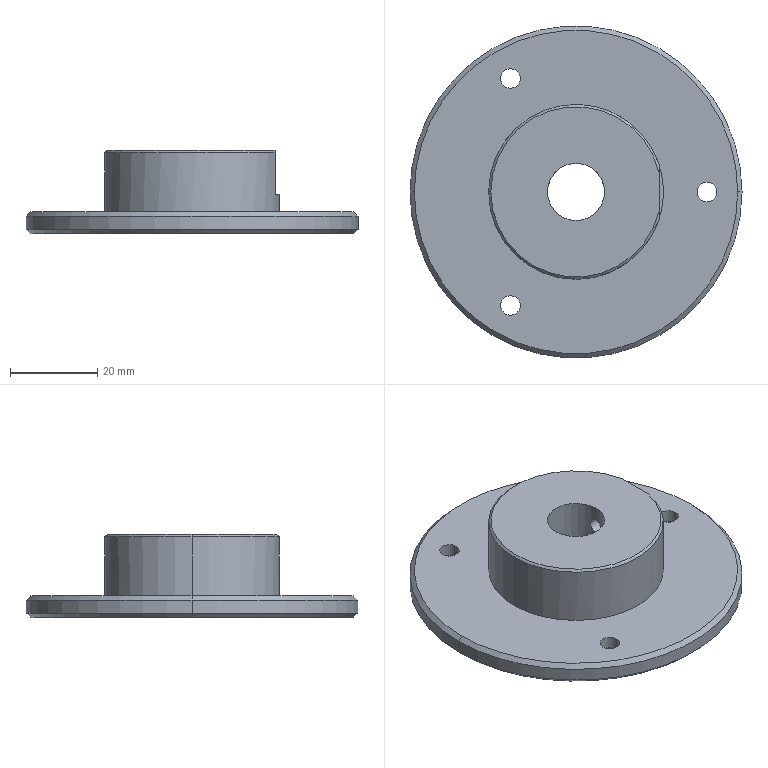Part | STEP file | 11-FG-B05411 | 1 solid | 31 faces | box 76 x 76 x 19 mm | volume 36918 mm3 | cylinder 14 | cone 12 | plane 5 | commonest cylinder face diameters 4.5 x6 3.3 x2 13.1 x2 40 x2 76 x2
STEP:
#1=CARTESIAN_POINT('',(-19.5,0.,19.));
#2=VERTEX_POINT('',#1);
#3=CARTESIAN_POINT('',(19.,-4.387,19.));
#4=VERTEX_POINT('',#3);
#5=CARTESIAN_POINT('',(0.,0.,19.));
#6=DIRECTION('',(0.,0.,1.));
#7=DIRECTION('',(1.,0.,0.));
#8=AXIS2_PLACEMENT_3D('',#5,#6,#7);
#9=CIRCLE('',#8,19.5);
#10=EDGE_CURVE('',#2,#4,#9,.T.);
#11=ORIENTED_EDGE('',*,*,#10,.F.);
#12=CARTESIAN_POINT('',(-20.,0.,18.5));
#13=VERTEX_POINT('',#12);
#14=CARTESIAN_POINT('',(-19.5,0.,19.));
#15=DIRECTION('',(-0.7071,0.,-0.7071));
#16=VECTOR('',#15,1000.);
#17=LINE('',#14,#16);
#18=EDGE_CURVE('',#2,#13,#17,.T.);
#19=ORIENTED_EDGE('',*,*,#18,.T.);
#20=CARTESIAN_POINT('',(19.,-6.245,18.5));
#21=VERTEX_POINT('',#20);
#22=CARTESIAN_POINT('',(0.,0.,18.5));
#23=DIRECTION('',(0.,0.,-1.));
#24=DIRECTION('',(1.,0.,0.));
#25=AXIS2_PLACEMENT_3D('',#22,#23,#24);
#26=CIRCLE('',#25,20.);
#27=EDGE_CURVE('',#21,#13,#26,.T.);
#28=ORIENTED_EDGE('',*,*,#27,.F.);
#29=CARTESIAN_POINT('',(19.,-4.387,19.));
#30=CARTESIAN_POINT('',(19.,-5.014,18.859));
#31=CARTESIAN_POINT('',(19.,-5.632,18.691));
#32=CARTESIAN_POINT('',(19.,-6.245,18.5));
#33=B_SPLINE_CURVE_WITH_KNOTS('',3,(#29,#30,#31,#32),.UNSPECIFIED.,.F.,.F.,(4,4),(0.,0.001924),.UNSPECIFIED.);
#34=EDGE_CURVE('',#4,#21,#33,.T.);
#35=ORIENTED_EDGE('',*,*,#34,.F.);
#36=EDGE_LOOP('',(#11,#19,#28,#35));
#37=FACE_OUTER_BOUND('',#36,.T.);
#38=CARTESIAN_POINT('',(0.,0.,19.));
#39=DIRECTION('',(0.,0.,-1.));
#40=DIRECTION('',(-1.,0.,0.));
#41=AXIS2_PLACEMENT_3D('',#38,#39,#40);
#42=CONICAL_SURFACE('',#41,19.5,0.7854);
#43=ADVANCED_FACE('',(#37),#42,.T.);
#44=CARTESIAN_POINT('',(6.55,0.,15.65));
#45=VERTEX_POINT('',#44);
#46=CARTESIAN_POINT('',(6.55,0.,12.35));
#47=VERTEX_POINT('',#46);
#48=CARTESIAN_POINT('',(6.55,0.,15.65));
#49=CARTESIAN_POINT('',(6.55,-0.2158,15.65));
#50=CARTESIAN_POINT('',(6.539,-0.4338,15.606));
#51=CARTESIAN_POINT('',(6.51,-0.7319,15.483));
#52=CARTESIAN_POINT('',(6.498,-0.8284,15.431));
#53=CARTESIAN_POINT('',(6.473,-1.007,15.311));
#54=CARTESIAN_POINT('',(6.459,-1.09,15.243));
#55=CARTESIAN_POINT('',(6.432,-1.242,15.091));
#56=CARTESIAN_POINT('',(6.418,-1.312,15.007));
#57=CARTESIAN_POINT('',(6.392,-1.431,14.829));
#58=CARTESIAN_POINT('',(6.38,-1.482,14.734));
#59=CARTESIAN_POINT('',(6.35,-1.607,14.433));
#60=CARTESIAN_POINT('',(6.339,-1.65,14.218));
#61=CARTESIAN_POINT('',(6.339,-1.65,13.892));
#62=CARTESIAN_POINT('',(6.342,-1.639,13.784));
#63=CARTESIAN_POINT('',(6.352,-1.597,13.572));
#64=CARTESIAN_POINT('',(6.36,-1.565,13.467));
#65=CARTESIAN_POINT('',(6.39,-1.441,13.169));
#66=CARTESIAN_POINT('',(6.418,-1.319,12.985));
#67=CARTESIAN_POINT('',(6.473,-1.016,12.682));
#68=CARTESIAN_POINT('',(6.5,-0.833,12.56));
#69=CARTESIAN_POINT('',(6.529,-0.5351,12.435));
#70=CARTESIAN_POINT('',(6.537,-0.43,12.403));
#71=CARTESIAN_POINT('',(6.547,-0.2173,12.361));
#72=CARTESIAN_POINT('',(6.55,-0.1095,12.35));
#73=CARTESIAN_POINT('',(6.55,0.,12.35));
#74=B_SPLINE_CURVE_WITH_KNOTS('',3,(#48,#49,#50,#51,#52,#53,#54,#55,#56,#57,#58,#59,#60,#61,#62,#63,#64,#65,#66,#67,#68,#69,#70,#71,#72,#73),.UNSPECIFIED.,.F.,.F.,(4,2,2,2,2,2,2,2,2,2,2,2,4),(0.00518,0.005827,0.006151,0.006474,0.006798,0.007121,0.007769,0.008092,0.008416,0.009063,0.009711,0.01003,0.01036),.UNSPECIFIED.);
#75=EDGE_CURVE('',#45,#47,#74,.T.);
#76=ORIENTED_EDGE('',*,*,#75,.F.);
#77=CARTESIAN_POINT('',(19.,0.,15.65));
#78=VERTEX_POINT('',#77);
#79=CARTESIAN_POINT('',(19.,0.,15.65));
#80=DIRECTION('',(1.,0.,0.));
#81=VECTOR('',#80,1000.);
#82=LINE('',#79,#81);
#83=EDGE_CURVE('',#45,#78,#82,.T.);
#84=ORIENTED_EDGE('',*,*,#83,.T.);
#85=CARTESIAN_POINT('',(19.,0.,12.35));
#86=VERTEX_POINT('',#85);
#87=CARTESIAN_POINT('',(19.,0.,14.));
#88=DIRECTION('',(1.,0.,0.));
#89=DIRECTION('',(0.,0.,-1.));
#90=AXIS2_PLACEMENT_3D('',#87,#88,#89);
#91=CIRCLE('',#90,1.65);
#92=EDGE_CURVE('',#78,#86,#91,.T.);
#93=ORIENTED_EDGE('',*,*,#92,.T.);
#94=CARTESIAN_POINT('',(19.,0.,12.35));
#95=DIRECTION('',(1.,0.,0.));
#96=VECTOR('',#95,1000.);
#97=LINE('',#94,#96);
#98=EDGE_CURVE('',#47,#86,#97,.T.);
#99=ORIENTED_EDGE('',*,*,#98,.F.);
#100=EDGE_LOOP('',(#76,#84,#93,#99));
#101=FACE_OUTER_BOUND('',#100,.T.);
#102=CARTESIAN_POINT('',(19.,0.,14.));
#103=DIRECTION('',(1.,0.,0.));
#104=DIRECTION('',(0.,0.,-1.));
#105=AXIS2_PLACEMENT_3D('',#102,#103,#104);
#106=CYLINDRICAL_SURFACE('',#105,1.65);
#107=ADVANCED_FACE('',(#101),#106,.F.);
#108=CARTESIAN_POINT('',(-12.75,25.981,2.05));
#109=VERTEX_POINT('',#108);
#110=CARTESIAN_POINT('',(-17.25,25.981,2.05));
#111=VERTEX_POINT('',#110);
#112=CARTESIAN_POINT('',(-15.,25.981,2.05));
#113=DIRECTION('',(0.,0.,-1.));
#114=DIRECTION('',(-1.,0.,0.));
#115=AXIS2_PLACEMENT_3D('',#112,#113,#114);
#116=CIRCLE('',#115,2.25);
#117=EDGE_CURVE('',#109,#111,#116,.T.);
#118=ORIENTED_EDGE('',*,*,#117,.F.);
#119=CARTESIAN_POINT('',(-10.7,25.981,0.));
#120=VERTEX_POINT('',#119);
#121=CARTESIAN_POINT('',(-10.7,25.981,0.));
#122=DIRECTION('',(0.7071,0.,-0.7071));
#123=VECTOR('',#122,1000.);
#124=LINE('',#121,#123);
#125=EDGE_CURVE('',#109,#120,#124,.T.);
#126=ORIENTED_EDGE('',*,*,#125,.T.);
#127=CARTESIAN_POINT('',(-19.3,25.981,0.));
#128=VERTEX_POINT('',#127);
#129=CARTESIAN_POINT('',(-15.,25.981,0.));
#130=DIRECTION('',(0.,0.,-1.));
#131=DIRECTION('',(-1.,0.,0.));
#132=AXIS2_PLACEMENT_3D('',#129,#130,#131);
#133=CIRCLE('',#132,4.3);
#134=EDGE_CURVE('',#120,#128,#133,.T.);
#135=ORIENTED_EDGE('',*,*,#134,.T.);
#136=CARTESIAN_POINT('',(-19.3,25.981,0.));
#137=DIRECTION('',(-0.7071,0.,-0.7071));
#138=VECTOR('',#137,1000.);
#139=LINE('',#136,#138);
#140=EDGE_CURVE('',#111,#128,#139,.T.);
#141=ORIENTED_EDGE('',*,*,#140,.F.);
#142=EDGE_LOOP('',(#118,#126,#135,#141));
#143=FACE_OUTER_BOUND('',#142,.T.);
#144=CARTESIAN_POINT('',(-15.,25.981,0.));
#145=DIRECTION('',(0.,0.,-1.));
#146=DIRECTION('',(-1.,0.,0.));
#147=AXIS2_PLACEMENT_3D('',#144,#145,#146);
#148=CONICAL_SURFACE('',#147,4.3,0.7854);
#149=ADVANCED_FACE('',(#143),#148,.F.);
#150=CARTESIAN_POINT('',(-17.25,25.981,5.));
#151=VERTEX_POINT('',#150);
#152=CARTESIAN_POINT('',(-12.75,25.981,5.));
#153=VERTEX_POINT('',#152);
#154=CARTESIAN_POINT('',(-15.,25.981,5.));
#155=DIRECTION('',(0.,0.,1.));
#156=DIRECTION('',(1.,0.,0.));
#157=AXIS2_PLACEMENT_3D('',#154,#155,#156);
#158=CIRCLE('',#157,2.25);
#159=EDGE_CURVE('',#151,#153,#158,.T.);
#160=ORIENTED_EDGE('',*,*,#159,.T.);
#161=CARTESIAN_POINT('',(-12.75,25.981,0.));
#162=DIRECTION('',(0.,0.,-1.));
#163=VECTOR('',#162,1000.);
#164=LINE('',#161,#163);
#165=EDGE_CURVE('',#153,#109,#164,.T.);
#166=ORIENTED_EDGE('',*,*,#165,.T.);
#167=ORIENTED_EDGE('',*,*,#117,.T.);
#168=CARTESIAN_POINT('',(-17.25,25.981,0.));
#169=DIRECTION('',(0.,0.,-1.));
#170=VECTOR('',#169,1000.);
#171=LINE('',#168,#170);
#172=EDGE_CURVE('',#151,#111,#171,.T.);
#173=ORIENTED_EDGE('',*,*,#172,.F.);
#174=EDGE_LOOP('',(#160,#166,#167,#173));
#175=FACE_OUTER_BOUND('',#174,.T.);
#176=CARTESIAN_POINT('',(-15.,25.981,0.));
#177=DIRECTION('',(0.,0.,-1.));
#178=DIRECTION('',(-1.,0.,0.));
#179=AXIS2_PLACEMENT_3D('',#176,#177,#178);
#180=CYLINDRICAL_SURFACE('',#179,2.25);
#181=ADVANCED_FACE('',(#175),#180,.F.);
#182=CARTESIAN_POINT('',(-12.75,-25.981,2.05));
#183=VERTEX_POINT('',#182);
#184=CARTESIAN_POINT('',(-17.25,-25.981,2.05));
#185=VERTEX_POINT('',#184);
#186=CARTESIAN_POINT('',(-15.,-25.981,2.05));
#187=DIRECTION('',(0.,0.,-1.));
#188=DIRECTION('',(-1.,0.,0.));
#189=AXIS2_PLACEMENT_3D('',#186,#187,#188);
#190=CIRCLE('',#189,2.25);
#191=EDGE_CURVE('',#183,#185,#190,.T.);
#192=ORIENTED_EDGE('',*,*,#191,.F.);
#193=CARTESIAN_POINT('',(-10.7,-25.981,0.));
#194=VERTEX_POINT('',#193);
#195=CARTESIAN_POINT('',(-10.7,-25.981,0.));
#196=DIRECTION('',(0.7071,0.,-0.7071));
#197=VECTOR('',#196,1000.);
#198=LINE('',#195,#197);
#199=EDGE_CURVE('',#183,#194,#198,.T.);
#200=ORIENTED_EDGE('',*,*,#199,.T.);
#201=CARTESIAN_POINT('',(-19.3,-25.981,0.));
#202=VERTEX_POINT('',#201);
#203=CARTESIAN_POINT('',(-15.,-25.981,0.));
#204=DIRECTION('',(0.,0.,-1.));
#205=DIRECTION('',(-1.,0.,0.));
#206=AXIS2_PLACEMENT_3D('',#203,#204,#205);
#207=CIRCLE('',#206,4.3);
#208=EDGE_CURVE('',#194,#202,#207,.T.);
#209=ORIENTED_EDGE('',*,*,#208,.T.);
#210=CARTESIAN_POINT('',(-19.3,-25.981,0.));
#211=DIRECTION('',(-0.7071,0.,-0.7071));
#212=VECTOR('',#211,1000.);
#213=LINE('',#210,#212);
#214=EDGE_CURVE('',#185,#202,#213,.T.);
#215=ORIENTED_EDGE('',*,*,#214,.F.);
#216=EDGE_LOOP('',(#192,#200,#209,#215));
#217=FACE_OUTER_BOUND('',#216,.T.);
#218=CARTESIAN_POINT('',(-15.,-25.981,0.));
#219=DIRECTION('',(0.,0.,-1.));
#220=DIRECTION('',(-1.,0.,0.));
#221=AXIS2_PLACEMENT_3D('',#218,#219,#220);
#222=CONICAL_SURFACE('',#221,4.3,0.7854);
#223=ADVANCED_FACE('',(#217),#222,.F.);
#224=CARTESIAN_POINT('',(-17.25,-25.981,5.));
#225=VERTEX_POINT('',#224);
#226=CARTESIAN_POINT('',(-12.75,-25.981,5.));
#227=VERTEX_POINT('',#226);
#228=CARTESIAN_POINT('',(-15.,-25.981,5.));
#229=DIRECTION('',(0.,0.,1.));
#230=DIRECTION('',(1.,0.,0.));
#231=AXIS2_PLACEMENT_3D('',#228,#229,#230);
#232=CIRCLE('',#231,2.25);
#233=EDGE_CURVE('',#225,#227,#232,.T.);
#234=ORIENTED_EDGE('',*,*,#233,.T.);
#235=CARTESIAN_POINT('',(-12.75,-25.981,0.));
#236=DIRECTION('',(0.,0.,-1.));
#237=VECTOR('',#236,1000.);
#238=LINE('',#235,#237);
#239=EDGE_CURVE('',#227,#183,#238,.T.);
#240=ORIENTED_EDGE('',*,*,#239,.T.);
#241=ORIENTED_EDGE('',*,*,#191,.T.);
#242=CARTESIAN_POINT('',(-17.25,-25.981,0.));
#243=DIRECTION('',(0.,0.,-1.));
#244=VECTOR('',#243,1000.);
#245=LINE('',#242,#244);
#246=EDGE_CURVE('',#225,#185,#245,.T.);
#247=ORIENTED_EDGE('',*,*,#246,.F.);
#248=EDGE_LOOP('',(#234,#240,#241,#247));
#249=FACE_OUTER_BOUND('',#248,.T.);
#250=CARTESIAN_POINT('',(-15.,-25.981,0.));
#251=DIRECTION('',(0.,0.,-1.));
#252=DIRECTION('',(-1.,0.,0.));
#253=AXIS2_PLACEMENT_3D('',#250,#251,#252);
#254=CYLINDRICAL_SURFACE('',#253,2.25);
#255=ADVANCED_FACE('',(#249),#254,.F.);
#256=CARTESIAN_POINT('',(32.25,0.,2.05));
#257=VERTEX_POINT('',#256);
#258=CARTESIAN_POINT('',(27.75,0.,2.05));
#259=VERTEX_POINT('',#258);
#260=CARTESIAN_POINT('',(30.,0.,2.05));
#261=DIRECTION('',(0.,0.,-1.));
#262=DIRECTION('',(-1.,0.,0.));
#263=AXIS2_PLACEMENT_3D('',#260,#261,#262);
#264=CIRCLE('',#263,2.25);
#265=EDGE_CURVE('',#257,#259,#264,.T.);
#266=ORIENTED_EDGE('',*,*,#265,.F.);
#267=CARTESIAN_POINT('',(34.3,0.,0.));
#268=VERTEX_POINT('',#267);
#269=CARTESIAN_POINT('',(34.3,0.,0.));
#270=DIRECTION('',(0.7071,0.,-0.7071));
#271=VECTOR('',#270,1000.);
#272=LINE('',#269,#271);
#273=EDGE_CURVE('',#257,#268,#272,.T.);
#274=ORIENTED_EDGE('',*,*,#273,.T.);
#275=CARTESIAN_POINT('',(25.7,0.,0.));
#276=VERTEX_POINT('',#275);
#277=CARTESIAN_POINT('',(30.,0.,0.));
#278=DIRECTION('',(0.,0.,-1.));
#279=DIRECTION('',(-1.,0.,0.));
#280=AXIS2_PLACEMENT_3D('',#277,#278,#279);
#281=CIRCLE('',#280,4.3);
#282=EDGE_CURVE('',#268,#276,#281,.T.);
#283=ORIENTED_EDGE('',*,*,#282,.T.);
#284=CARTESIAN_POINT('',(25.7,0.,0.));
#285=DIRECTION('',(-0.7071,0.,-0.7071));
#286=VECTOR('',#285,1000.);
#287=LINE('',#284,#286);
#288=EDGE_CURVE('',#259,#276,#287,.T.);
#289=ORIENTED_EDGE('',*,*,#288,.F.);
#290=EDGE_LOOP('',(#266,#274,#283,#289));
#291=FACE_OUTER_BOUND('',#290,.T.);
#292=CARTESIAN_POINT('',(30.,0.,0.));
#293=DIRECTION('',(0.,0.,-1.));
#294=DIRECTION('',(-1.,0.,0.));
#295=AXIS2_PLACEMENT_3D('',#292,#293,#294);
#296=CONICAL_SURFACE('',#295,4.3,0.7854);
#297=ADVANCED_FACE('',(#291),#296,.F.);
#298=CARTESIAN_POINT('',(27.75,0.,5.));
#299=VERTEX_POINT('',#298);
#300=CARTESIAN_POINT('',(32.25,0.,5.));
#301=VERTEX_POINT('',#300);
#302=CARTESIAN_POINT('',(30.,0.,5.));
#303=DIRECTION('',(0.,0.,1.));
#304=DIRECTION('',(1.,0.,0.));
#305=AXIS2_PLACEMENT_3D('',#302,#303,#304);
#306=CIRCLE('',#305,2.25);
#307=EDGE_CURVE('',#299,#301,#306,.T.);
#308=ORIENTED_EDGE('',*,*,#307,.T.);
#309=CARTESIAN_POINT('',(32.25,0.,0.));
#310=DIRECTION('',(0.,0.,-1.));
#311=VECTOR('',#310,1000.);
#312=LINE('',#309,#311);
#313=EDGE_CURVE('',#301,#257,#312,.T.);
#314=ORIENTED_EDGE('',*,*,#313,.T.);
#315=ORIENTED_EDGE('',*,*,#265,.T.);
#316=CARTESIAN_POINT('',(27.75,0.,0.));
#317=DIRECTION('',(0.,0.,-1.));
#318=VECTOR('',#317,1000.);
#319=LINE('',#316,#318);
#320=EDGE_CURVE('',#299,#259,#319,.T.);
#321=ORIENTED_EDGE('',*,*,#320,.F.);
#322=EDGE_LOOP('',(#308,#314,#315,#321));
#323=FACE_OUTER_BOUND('',#322,.T.);
#324=CARTESIAN_POINT('',(30.,0.,0.));
#325=DIRECTION('',(0.,0.,-1.));
#326=DIRECTION('',(-1.,0.,0.));
#327=AXIS2_PLACEMENT_3D('',#324,#325,#326);
#328=CYLINDRICAL_SURFACE('',#327,2.25);
#329=ADVANCED_FACE('',(#323),#328,.F.);
#330=CARTESIAN_POINT('',(6.55,0.,19.));
#331=VERTEX_POINT('',#330);
#332=CARTESIAN_POINT('',(-6.55,0.,19.));
#333=VERTEX_POINT('',#332);
#334=CARTESIAN_POINT('',(0.,0.,19.));
#335=DIRECTION('',(0.,0.,-1.));
#336=DIRECTION('',(-1.,0.,0.));
#337=AXIS2_PLACEMENT_3D('',#334,#335,#336);
#338=CIRCLE('',#337,6.55);
#339=EDGE_CURVE('',#331,#333,#338,.T.);
#340=ORIENTED_EDGE('',*,*,#339,.F.);
#341=CARTESIAN_POINT('',(6.55,0.,19.));
#342=DIRECTION('',(0.,0.,-1.));
#343=VECTOR('',#342,1000.);
#344=LINE('',#341,#343);
#345=EDGE_CURVE('',#331,#45,#344,.T.);
#346=ORIENTED_EDGE('',*,*,#345,.T.);
#347=ORIENTED_EDGE('',*,*,#75,.T.);
#348=CARTESIAN_POINT('',(6.55,0.,0.));
#349=VERTEX_POINT('',#348);
#350=CARTESIAN_POINT('',(6.55,0.,19.));
#351=DIRECTION('',(0.,0.,-1.));
#352=VECTOR('',#351,1000.);
#353=LINE('',#350,#352);
#354=EDGE_CURVE('',#47,#349,#353,.T.);
#355=ORIENTED_EDGE('',*,*,#354,.T.);
#356=CARTESIAN_POINT('',(-6.55,0.,0.));
#357=VERTEX_POINT('',#356);
#358=CARTESIAN_POINT('',(0.,0.,0.));
#359=DIRECTION('',(0.,0.,-1.));
#360=DIRECTION('',(-1.,0.,0.));
#361=AXIS2_PLACEMENT_3D('',#358,#359,#360);
#362=CIRCLE('',#361,6.55);
#363=EDGE_CURVE('',#349,#357,#362,.T.);
#364=ORIENTED_EDGE('',*,*,#363,.T.);
#365=CARTESIAN_POINT('',(-6.55,0.,19.));
#366=DIRECTION('',(0.,0.,-1.));
#367=VECTOR('',#366,1000.);
#368=LINE('',#365,#367);
#369=EDGE_CURVE('',#333,#357,#368,.T.);
#370=ORIENTED_EDGE('',*,*,#369,.F.);
#371=EDGE_LOOP('',(#340,#346,#347,#355,#364,#370));
#372=FACE_OUTER_BOUND('',#371,.T.);
#373=CARTESIAN_POINT('',(0.,0.,19.));
#374=DIRECTION('',(0.,0.,-1.));
#375=DIRECTION('',(-1.,0.,0.));
#376=AXIS2_PLACEMENT_3D('',#373,#374,#375);
#377=CYLINDRICAL_SURFACE('',#376,6.55);
#378=ADVANCED_FACE('',(#372),#377,.F.);
#379=CARTESIAN_POINT('',(-37.,0.,0.));
#380=VERTEX_POINT('',#379);
#381=CARTESIAN_POINT('',(37.,0.,0.));
#382=VERTEX_POINT('',#381);
#383=CARTESIAN_POINT('',(0.,0.,0.));
#384=DIRECTION('',(0.,0.,-1.));
#385=DIRECTION('',(1.,0.,0.));
#386=AXIS2_PLACEMENT_3D('',#383,#384,#385);
#387=CIRCLE('',#386,37.);
#388=EDGE_CURVE('',#380,#382,#387,.T.);
#389=ORIENTED_EDGE('',*,*,#388,.F.);
#390=CARTESIAN_POINT('',(-38.,0.,1.));
#391=VERTEX_POINT('',#390);
#392=CARTESIAN_POINT('',(-38.,0.,1.));
#393=DIRECTION('',(-0.7071,0.,0.7071));
#394=VECTOR('',#393,1000.);
#395=LINE('',#392,#394);
#396=EDGE_CURVE('',#380,#391,#395,.T.);
#397=ORIENTED_EDGE('',*,*,#396,.T.);
#398=CARTESIAN_POINT('',(38.,0.,1.));
#399=VERTEX_POINT('',#398);
#400=CARTESIAN_POINT('',(0.,0.,1.));
#401=DIRECTION('',(0.,0.,1.));
#402=DIRECTION('',(1.,0.,0.));
#403=AXIS2_PLACEMENT_3D('',#400,#401,#402);
#404=CIRCLE('',#403,38.);
#405=EDGE_CURVE('',#399,#391,#404,.T.);
#406=ORIENTED_EDGE('',*,*,#405,.F.);
#407=CARTESIAN_POINT('',(38.,0.,1.));
#408=DIRECTION('',(0.7071,0.,0.7071));
#409=VECTOR('',#408,1000.);
#410=LINE('',#407,#409);
#411=EDGE_CURVE('',#382,#399,#410,.T.);
#412=ORIENTED_EDGE('',*,*,#411,.F.);
#413=EDGE_LOOP('',(#389,#397,#406,#412));
#414=FACE_OUTER_BOUND('',#413,.T.);
#415=CARTESIAN_POINT('',(0.,0.,1.));
#416=DIRECTION('',(0.,0.,1.));
#417=DIRECTION('',(1.,0.,0.));
#418=AXIS2_PLACEMENT_3D('',#415,#416,#417);
#419=CONICAL_SURFACE('',#418,38.,0.7854);
#420=ADVANCED_FACE('',(#414),#419,.T.);
#421=CARTESIAN_POINT('',(37.,0.,5.));
#422=VERTEX_POINT('',#421);
#423=CARTESIAN_POINT('',(-37.,0.,5.));
#424=VERTEX_POINT('',#423);
#425=CARTESIAN_POINT('',(0.,0.,5.));
#426=DIRECTION('',(0.,0.,1.));
#427=DIRECTION('',(1.,0.,0.));
#428=AXIS2_PLACEMENT_3D('',#425,#426,#427);
#429=CIRCLE('',#428,37.);
#430=EDGE_CURVE('',#422,#424,#429,.T.);
#431=ORIENTED_EDGE('',*,*,#430,.F.);
#432=CARTESIAN_POINT('',(38.,0.,4.));
#433=VERTEX_POINT('',#432);
#434=CARTESIAN_POINT('',(37.,0.,5.));
#435=DIRECTION('',(0.7071,0.,-0.7071));
#436=VECTOR('',#435,1000.);
#437=LINE('',#434,#436);
#438=EDGE_CURVE('',#422,#433,#437,.T.);
#439=ORIENTED_EDGE('',*,*,#438,.T.);
#440=CARTESIAN_POINT('',(-38.,0.,4.));
#441=VERTEX_POINT('',#440);
#442=CARTESIAN_POINT('',(0.,0.,4.));
#443=DIRECTION('',(0.,0.,-1.));
#444=DIRECTION('',(1.,0.,0.));
#445=AXIS2_PLACEMENT_3D('',#442,#443,#444);
#446=CIRCLE('',#445,38.);
#447=EDGE_CURVE('',#441,#433,#446,.T.);
#448=ORIENTED_EDGE('',*,*,#447,.F.);
#449=CARTESIAN_POINT('',(-37.,0.,5.));
#450=DIRECTION('',(-0.7071,0.,-0.7071));
#451=VECTOR('',#450,1000.);
#452=LINE('',#449,#451);
#453=EDGE_CURVE('',#424,#441,#452,.T.);
#454=ORIENTED_EDGE('',*,*,#453,.F.);
#455=EDGE_LOOP('',(#431,#439,#448,#454));
#456=FACE_OUTER_BOUND('',#455,.T.);
#457=CARTESIAN_POINT('',(0.,0.,5.));
#458=DIRECTION('',(0.,0.,-1.));
#459=DIRECTION('',(-1.,0.,0.));
#460=AXIS2_PLACEMENT_3D('',#457,#458,#459);
#461=CONICAL_SURFACE('',#460,37.,0.7854);
#462=ADVANCED_FACE('',(#456),#461,.T.);
#463=CARTESIAN_POINT('',(20.,0.,9.));
#464=VERTEX_POINT('',#463);
#465=CARTESIAN_POINT('',(19.,6.245,9.));
#466=VERTEX_POINT('',#465);
#467=CARTESIAN_POINT('',(0.,0.,9.));
#468=DIRECTION('',(0.,0.,1.));
#469=DIRECTION('',(1.,0.,0.));
#470=AXIS2_PLACEMENT_3D('',#467,#468,#469);
#471=CIRCLE('',#470,20.);
#472=EDGE_CURVE('',#464,#466,#471,.T.);
#473=ORIENTED_EDGE('',*,*,#472,.F.);
#474=CARTESIAN_POINT('',(20.,0.,5.));
#475=VERTEX_POINT('',#474);
#476=CARTESIAN_POINT('',(20.,0.,19.));
#477=DIRECTION('',(0.,0.,-1.));
#478=VECTOR('',#477,1000.);
#479=LINE('',#476,#478);
#480=EDGE_CURVE('',#464,#475,#479,.T.);
#481=ORIENTED_EDGE('',*,*,#480,.T.);
#482=CARTESIAN_POINT('',(-20.,0.,5.));
#483=VERTEX_POINT('',#482);
#484=CARTESIAN_POINT('',(0.,0.,5.));
#485=DIRECTION('',(0.,0.,1.));
#486=DIRECTION('',(1.,0.,0.));
#487=AXIS2_PLACEMENT_3D('',#484,#485,#486);
#488=CIRCLE('',#487,20.);
#489=EDGE_CURVE('',#475,#483,#488,.T.);
#490=ORIENTED_EDGE('',*,*,#489,.T.);
#491=CARTESIAN_POINT('',(-20.,0.,19.));
#492=DIRECTION('',(0.,0.,-1.));
#493=VECTOR('',#492,1000.);
#494=LINE('',#491,#493);
#495=EDGE_CURVE('',#13,#483,#494,.T.);
#496=ORIENTED_EDGE('',*,*,#495,.F.);
#497=CARTESIAN_POINT('',(19.,6.245,18.5));
#498=VERTEX_POINT('',#497);
#499=CARTESIAN_POINT('',(0.,0.,18.5));
#500=DIRECTION('',(0.,0.,-1.));
#501=DIRECTION('',(1.,0.,0.));
#502=AXIS2_PLACEMENT_3D('',#499,#500,#501);
#503=CIRCLE('',#502,20.);
#504=EDGE_CURVE('',#13,#498,#503,.T.);
#505=ORIENTED_EDGE('',*,*,#504,.T.);
#506=CARTESIAN_POINT('',(19.,6.245,19.));
#507=DIRECTION('',(0.,0.,-1.));
#508=VECTOR('',#507,1000.);
#509=LINE('',#506,#508);
#510=EDGE_CURVE('',#498,#466,#509,.T.);
#511=ORIENTED_EDGE('',*,*,#510,.T.);
#512=EDGE_LOOP('',(#473,#481,#490,#496,#505,#511));
#513=FACE_OUTER_BOUND('',#512,.T.);
#514=CARTESIAN_POINT('',(0.,0.,19.));
#515=DIRECTION('',(0.,0.,-1.));
#516=DIRECTION('',(-1.,0.,0.));
#517=AXIS2_PLACEMENT_3D('',#514,#515,#516);
#518=CYLINDRICAL_SURFACE('',#517,20.);
#519=ADVANCED_FACE('',(#513),#518,.T.);
#520=ORIENTED_EDGE('',*,*,#447,.T.);
#521=CARTESIAN_POINT('',(38.,0.,5.));
#522=DIRECTION('',(0.,0.,-1.));
#523=VECTOR('',#522,1000.);
#524=LINE('',#521,#523);
#525=EDGE_CURVE('',#433,#399,#524,.T.);
#526=ORIENTED_EDGE('',*,*,#525,.T.);
#527=ORIENTED_EDGE('',*,*,#405,.T.);
#528=CARTESIAN_POINT('',(-38.,0.,5.));
#529=DIRECTION('',(0.,0.,-1.));
#530=VECTOR('',#529,1000.);
#531=LINE('',#528,#530);
#532=EDGE_CURVE('',#441,#391,#531,.T.);
#533=ORIENTED_EDGE('',*,*,#532,.F.);
#534=EDGE_LOOP('',(#520,#526,#527,#533));
#535=FACE_OUTER_BOUND('',#534,.T.);
#536=CARTESIAN_POINT('',(0.,0.,5.));
#537=DIRECTION('',(0.,0.,-1.));
#538=DIRECTION('',(-1.,0.,0.));
#539=AXIS2_PLACEMENT_3D('',#536,#537,#538);
#540=CYLINDRICAL_SURFACE('',#539,38.);
#541=ADVANCED_FACE('',(#535),#540,.T.);
#542=ORIENTED_EDGE('',*,*,#159,.F.);
#543=CARTESIAN_POINT('',(-15.,25.981,5.));
#544=DIRECTION('',(0.,0.,1.));
#545=DIRECTION('',(1.,0.,0.));
#546=AXIS2_PLACEMENT_3D('',#543,#544,#545);
#547=CIRCLE('',#546,2.25);
#548=EDGE_CURVE('',#153,#151,#547,.T.);
#549=ORIENTED_EDGE('',*,*,#548,.F.);
#550=EDGE_LOOP('',(#542,#549));
#551=FACE_BOUND('',#550,.T.);
#552=ORIENTED_EDGE('',*,*,#233,.F.);
#553=CARTESIAN_POINT('',(-15.,-25.981,5.));
#554=DIRECTION('',(0.,0.,1.));
#555=DIRECTION('',(1.,0.,0.));
#556=AXIS2_PLACEMENT_3D('',#553,#554,#555);
#557=CIRCLE('',#556,2.25);
#558=EDGE_CURVE('',#227,#225,#557,.T.);
#559=ORIENTED_EDGE('',*,*,#558,.F.);
#560=EDGE_LOOP('',(#552,#559));
#561=FACE_BOUND('',#560,.T.);
#562=ORIENTED_EDGE('',*,*,#307,.F.);
#563=CARTESIAN_POINT('',(30.,0.,5.));
#564=DIRECTION('',(0.,0.,1.));
#565=DIRECTION('',(1.,0.,0.));
#566=AXIS2_PLACEMENT_3D('',#563,#564,#565);
#567=CIRCLE('',#566,2.25);
#568=EDGE_CURVE('',#301,#299,#567,.T.);
#569=ORIENTED_EDGE('',*,*,#568,.F.);
#570=EDGE_LOOP('',(#562,#569));
#571=FACE_BOUND('',#570,.T.);
#572=CARTESIAN_POINT('',(0.,0.,5.));
#573=DIRECTION('',(0.,0.,1.));
#574=DIRECTION('',(1.,0.,0.));
#575=AXIS2_PLACEMENT_3D('',#572,#573,#574);
#576=CIRCLE('',#575,37.);
#577=EDGE_CURVE('',#424,#422,#576,.T.);
#578=ORIENTED_EDGE('',*,*,#577,.T.);
#579=ORIENTED_EDGE('',*,*,#430,.T.);
#580=EDGE_LOOP('',(#578,#579));
#581=FACE_OUTER_BOUND('',#580,.T.);
#582=CARTESIAN_POINT('',(0.,0.,5.));
#583=DIRECTION('',(0.,0.,1.));
#584=DIRECTION('',(1.,0.,0.));
#585=AXIS2_PLACEMENT_3D('',#582,#583,#584);
#586=CIRCLE('',#585,20.);
#587=EDGE_CURVE('',#483,#475,#586,.T.);
#588=ORIENTED_EDGE('',*,*,#587,.F.);
#589=ORIENTED_EDGE('',*,*,#489,.F.);
#590=EDGE_LOOP('',(#588,#589));
#591=FACE_BOUND('',#590,.T.);
#592=CARTESIAN_POINT('',(0.,0.,5.));
#593=DIRECTION('',(0.,0.,1.));
#594=DIRECTION('',(1.,0.,0.));
#595=AXIS2_PLACEMENT_3D('',#592,#593,#594);
#596=PLANE('',#595);
#597=ADVANCED_FACE('',(#551,#561,#571,#581,#591),#596,.T.);
#598=ORIENTED_EDGE('',*,*,#525,.F.);
#599=CARTESIAN_POINT('',(0.,0.,4.));
#600=DIRECTION('',(0.,0.,-1.));
#601=DIRECTION('',(1.,0.,0.));
#602=AXIS2_PLACEMENT_3D('',#599,#600,#601);
#603=CIRCLE('',#602,38.);
#604=EDGE_CURVE('',#433,#441,#603,.T.);
#605=ORIENTED_EDGE('',*,*,#604,.T.);
#606=ORIENTED_EDGE('',*,*,#532,.T.);
#607=CARTESIAN_POINT('',(0.,0.,1.));
#608=DIRECTION('',(0.,0.,1.));
#609=DIRECTION('',(1.,0.,0.));
#610=AXIS2_PLACEMENT_3D('',#607,#608,#609);
#611=CIRCLE('',#610,38.);
#612=EDGE_CURVE('',#391,#399,#611,.T.);
#613=ORIENTED_EDGE('',*,*,#612,.T.);
#614=EDGE_LOOP('',(#598,#605,#606,#613));
#615=FACE_OUTER_BOUND('',#614,.T.);
#616=CARTESIAN_POINT('',(0.,0.,5.));
#617=DIRECTION('',(0.,0.,-1.));
#618=DIRECTION('',(-1.,0.,0.));
#619=AXIS2_PLACEMENT_3D('',#616,#617,#618);
#620=CYLINDRICAL_SURFACE('',#619,38.);
#621=ADVANCED_FACE('',(#615),#620,.T.);
#622=CARTESIAN_POINT('',(-15.,25.981,0.));
#623=DIRECTION('',(0.,0.,-1.));
#624=DIRECTION('',(-1.,0.,0.));
#625=AXIS2_PLACEMENT_3D('',#622,#623,#624);
#626=CIRCLE('',#625,4.3);
#627=EDGE_CURVE('',#128,#120,#626,.T.);
#628=ORIENTED_EDGE('',*,*,#627,.F.);
#629=ORIENTED_EDGE('',*,*,#134,.F.);
#630=EDGE_LOOP('',(#628,#629));
#631=FACE_BOUND('',#630,.T.);
#632=CARTESIAN_POINT('',(-15.,-25.981,0.));
#633=DIRECTION('',(0.,0.,-1.));
#634=DIRECTION('',(-1.,0.,0.));
#635=AXIS2_PLACEMENT_3D('',#632,#633,#634);
#636=CIRCLE('',#635,4.3);
#637=EDGE_CURVE('',#202,#194,#636,.T.);
#638=ORIENTED_EDGE('',*,*,#637,.F.);
#639=ORIENTED_EDGE('',*,*,#208,.F.);
#640=EDGE_LOOP('',(#638,#639));
#641=FACE_BOUND('',#640,.T.);
#642=CARTESIAN_POINT('',(30.,0.,0.));
#643=DIRECTION('',(0.,0.,-1.));
#644=DIRECTION('',(-1.,0.,0.));
#645=AXIS2_PLACEMENT_3D('',#642,#643,#644);
#646=CIRCLE('',#645,4.3);
#647=EDGE_CURVE('',#276,#268,#646,.T.);
#648=ORIENTED_EDGE('',*,*,#647,.F.);
#649=ORIENTED_EDGE('',*,*,#282,.F.);
#650=EDGE_LOOP('',(#648,#649));
#651=FACE_BOUND('',#650,.T.);
#652=CARTESIAN_POINT('',(0.,0.,0.));
#653=DIRECTION('',(0.,0.,-1.));
#654=DIRECTION('',(-1.,0.,0.));
#655=AXIS2_PLACEMENT_3D('',#652,#653,#654);
#656=CIRCLE('',#655,6.55);
#657=EDGE_CURVE('',#357,#349,#656,.T.);
#658=ORIENTED_EDGE('',*,*,#657,.F.);
#659=ORIENTED_EDGE('',*,*,#363,.F.);
#660=EDGE_LOOP('',(#658,#659));
#661=FACE_BOUND('',#660,.T.);
#662=CARTESIAN_POINT('',(0.,0.,0.));
#663=DIRECTION('',(0.,0.,-1.));
#664=DIRECTION('',(1.,0.,0.));
#665=AXIS2_PLACEMENT_3D('',#662,#663,#664);
#666=CIRCLE('',#665,37.);
#667=EDGE_CURVE('',#382,#380,#666,.T.);
#668=ORIENTED_EDGE('',*,*,#667,.T.);
#669=ORIENTED_EDGE('',*,*,#388,.T.);
#670=EDGE_LOOP('',(#668,#669));
#671=FACE_OUTER_BOUND('',#670,.T.);
#672=CARTESIAN_POINT('',(0.,0.,0.));
#673=DIRECTION('',(0.,0.,1.));
#674=DIRECTION('',(1.,0.,0.));
#675=AXIS2_PLACEMENT_3D('',#672,#673,#674);
#676=PLANE('',#675);
#677=ADVANCED_FACE('',(#631,#641,#651,#661,#671),#676,.F.);
#678=ORIENTED_EDGE('',*,*,#480,.F.);
#679=CARTESIAN_POINT('',(19.,-6.245,9.));
#680=VERTEX_POINT('',#679);
#681=CARTESIAN_POINT('',(0.,0.,9.));
#682=DIRECTION('',(0.,0.,1.));
#683=DIRECTION('',(1.,0.,0.));
#684=AXIS2_PLACEMENT_3D('',#681,#682,#683);
#685=CIRCLE('',#684,20.);
#686=EDGE_CURVE('',#680,#464,#685,.T.);
#687=ORIENTED_EDGE('',*,*,#686,.F.);
#688=CARTESIAN_POINT('',(19.,-6.245,19.));
#689=DIRECTION('',(0.,0.,1.));
#690=VECTOR('',#689,1000.);
#691=LINE('',#688,#690);
#692=EDGE_CURVE('',#680,#21,#691,.T.);
#693=ORIENTED_EDGE('',*,*,#692,.T.);
#694=ORIENTED_EDGE('',*,*,#27,.T.);
#695=ORIENTED_EDGE('',*,*,#495,.T.);
#696=ORIENTED_EDGE('',*,*,#587,.T.);
#697=EDGE_LOOP('',(#678,#687,#693,#694,#695,#696));
#698=FACE_OUTER_BOUND('',#697,.T.);
#699=CARTESIAN_POINT('',(0.,0.,19.));
#700=DIRECTION('',(0.,0.,-1.));
#701=DIRECTION('',(-1.,0.,0.));
#702=AXIS2_PLACEMENT_3D('',#699,#700,#701);
#703=CYLINDRICAL_SURFACE('',#702,20.);
#704=ADVANCED_FACE('',(#698),#703,.T.);
#705=CARTESIAN_POINT('',(19.,4.387,19.));
#706=VERTEX_POINT('',#705);
#707=CARTESIAN_POINT('',(19.,0.,19.));
#708=DIRECTION('',(0.,-1.,0.));
#709=VECTOR('',#708,1000.);
#710=LINE('',#707,#709);
#711=EDGE_CURVE('',#706,#4,#710,.T.);
#712=ORIENTED_EDGE('',*,*,#711,.F.);
#713=CARTESIAN_POINT('',(0.,0.,19.));
#714=DIRECTION('',(0.,0.,1.));
#715=DIRECTION('',(1.,0.,0.));
#716=AXIS2_PLACEMENT_3D('',#713,#714,#715);
#717=CIRCLE('',#716,19.5);
#718=EDGE_CURVE('',#706,#2,#717,.T.);
#719=ORIENTED_EDGE('',*,*,#718,.T.);
#720=ORIENTED_EDGE('',*,*,#10,.T.);
#721=EDGE_LOOP('',(#712,#719,#720));
#722=FACE_OUTER_BOUND('',#721,.T.);
#723=CARTESIAN_POINT('',(0.,0.,19.));
#724=DIRECTION('',(0.,0.,-1.));
#725=DIRECTION('',(-1.,0.,0.));
#726=AXIS2_PLACEMENT_3D('',#723,#724,#725);
#727=CIRCLE('',#726,6.55);
#728=EDGE_CURVE('',#333,#331,#727,.T.);
#729=ORIENTED_EDGE('',*,*,#728,.T.);
#730=ORIENTED_EDGE('',*,*,#339,.T.);
#731=EDGE_LOOP('',(#729,#730));
#732=FACE_BOUND('',#731,.T.);
#733=CARTESIAN_POINT('',(0.,0.,19.));
#734=DIRECTION('',(0.,0.,1.));
#735=DIRECTION('',(1.,0.,0.));
#736=AXIS2_PLACEMENT_3D('',#733,#734,#735);
#737=PLANE('',#736);
#738=ADVANCED_FACE('',(#722,#732),#737,.T.);
#739=ORIENTED_EDGE('',*,*,#438,.F.);
#740=ORIENTED_EDGE('',*,*,#577,.F.);
#741=ORIENTED_EDGE('',*,*,#453,.T.);
#742=ORIENTED_EDGE('',*,*,#604,.F.);
#743=EDGE_LOOP('',(#739,#740,#741,#742));
#744=FACE_OUTER_BOUND('',#743,.T.);
#745=CARTESIAN_POINT('',(0.,0.,5.));
#746=DIRECTION('',(0.,0.,-1.));
#747=DIRECTION('',(-1.,0.,0.));
#748=AXIS2_PLACEMENT_3D('',#745,#746,#747);
#749=CONICAL_SURFACE('',#748,37.,0.7854);
#750=ADVANCED_FACE('',(#744),#749,.T.);
#751=ORIENTED_EDGE('',*,*,#396,.F.);
#752=ORIENTED_EDGE('',*,*,#667,.F.);
#753=ORIENTED_EDGE('',*,*,#411,.T.);
#754=ORIENTED_EDGE('',*,*,#612,.F.);
#755=EDGE_LOOP('',(#751,#752,#753,#754));
#756=FACE_OUTER_BOUND('',#755,.T.);
#757=CARTESIAN_POINT('',(0.,0.,1.));
#758=DIRECTION('',(0.,0.,1.));
#759=DIRECTION('',(1.,0.,0.));
#760=AXIS2_PLACEMENT_3D('',#757,#758,#759);
#761=CONICAL_SURFACE('',#760,38.,0.7854);
#762=ADVANCED_FACE('',(#756),#761,.T.);
#763=ORIENTED_EDGE('',*,*,#345,.F.);
#764=ORIENTED_EDGE('',*,*,#728,.F.);
#765=ORIENTED_EDGE('',*,*,#369,.T.);
#766=ORIENTED_EDGE('',*,*,#657,.T.);
#767=ORIENTED_EDGE('',*,*,#354,.F.);
#768=CARTESIAN_POINT('',(6.55,0.,12.35));
#769=CARTESIAN_POINT('',(6.55,0.1095,12.35));
#770=CARTESIAN_POINT('',(6.547,0.2171,12.361));
#771=CARTESIAN_POINT('',(6.537,0.4286,12.403));
#772=CARTESIAN_POINT('',(6.529,0.5336,12.435));
#773=CARTESIAN_POINT('',(6.51,0.7333,12.518));
#774=CARTESIAN_POINT('',(6.498,0.8279,12.569));
#775=CARTESIAN_POINT('',(6.473,1.007,12.688));
#776=CARTESIAN_POINT('',(6.459,1.091,12.758));
#777=CARTESIAN_POINT('',(6.418,1.319,12.985));
#778=CARTESIAN_POINT('',(6.39,1.441,13.169));
#779=CARTESIAN_POINT('',(6.351,1.606,13.565));
#780=CARTESIAN_POINT('',(6.339,1.65,13.783));
#781=CARTESIAN_POINT('',(6.339,1.65,14.107));
#782=CARTESIAN_POINT('',(6.342,1.639,14.217));
#783=CARTESIAN_POINT('',(6.352,1.597,14.429));
#784=CARTESIAN_POINT('',(6.36,1.566,14.532));
#785=CARTESIAN_POINT('',(6.39,1.441,14.833));
#786=CARTESIAN_POINT('',(6.418,1.319,15.014));
#787=CARTESIAN_POINT('',(6.459,1.09,15.243));
#788=CARTESIAN_POINT('',(6.473,1.007,15.311));
#789=CARTESIAN_POINT('',(6.498,0.8288,15.431));
#790=CARTESIAN_POINT('',(6.51,0.7321,15.483));
#791=CARTESIAN_POINT('',(6.529,0.5329,15.565));
#792=CARTESIAN_POINT('',(6.537,0.43,15.597));
#793=CARTESIAN_POINT('',(6.547,0.2175,15.639));
#794=CARTESIAN_POINT('',(6.55,0.1079,15.65));
#795=CARTESIAN_POINT('',(6.55,0.,15.65));
#796=B_SPLINE_CURVE_WITH_KNOTS('',3,(#768,#769,#770,#771,#772,#773,#774,#775,#776,#777,#778,#779,#780,#781,#782,#783,#784,#785,#786,#787,#788,#789,#790,#791,#792,#793,#794,#795),.UNSPECIFIED.,.F.,.F.,(4,2,2,2,2,2,2,2,2,2,2,2,2,4),(0.,0.0003237,0.0006474,0.0009712,0.001295,0.001942,0.00259,0.002914,0.003237,0.003885,0.004208,0.004532,0.004856,0.00518),.UNSPECIFIED.);
#797=EDGE_CURVE('',#47,#45,#796,.T.);
#798=ORIENTED_EDGE('',*,*,#797,.T.);
#799=EDGE_LOOP('',(#763,#764,#765,#766,#767,#798));
#800=FACE_OUTER_BOUND('',#799,.T.);
#801=CARTESIAN_POINT('',(0.,0.,19.));
#802=DIRECTION('',(0.,0.,-1.));
#803=DIRECTION('',(-1.,0.,0.));
#804=AXIS2_PLACEMENT_3D('',#801,#802,#803);
#805=CYLINDRICAL_SURFACE('',#804,6.55);
#806=ADVANCED_FACE('',(#800),#805,.F.);
#807=ORIENTED_EDGE('',*,*,#313,.F.);
#808=ORIENTED_EDGE('',*,*,#568,.T.);
#809=ORIENTED_EDGE('',*,*,#320,.T.);
#810=CARTESIAN_POINT('',(30.,0.,2.05));
#811=DIRECTION('',(0.,0.,-1.));
#812=DIRECTION('',(-1.,0.,0.));
#813=AXIS2_PLACEMENT_3D('',#810,#811,#812);
#814=CIRCLE('',#813,2.25);
#815=EDGE_CURVE('',#259,#257,#814,.T.);
#816=ORIENTED_EDGE('',*,*,#815,.T.);
#817=EDGE_LOOP('',(#807,#808,#809,#816));
#818=FACE_OUTER_BOUND('',#817,.T.);
#819=CARTESIAN_POINT('',(30.,0.,0.));
#820=DIRECTION('',(0.,0.,-1.));
#821=DIRECTION('',(-1.,0.,0.));
#822=AXIS2_PLACEMENT_3D('',#819,#820,#821);
#823=CYLINDRICAL_SURFACE('',#822,2.25);
#824=ADVANCED_FACE('',(#818),#823,.F.);
#825=ORIENTED_EDGE('',*,*,#273,.F.);
#826=ORIENTED_EDGE('',*,*,#815,.F.);
#827=ORIENTED_EDGE('',*,*,#288,.T.);
#828=ORIENTED_EDGE('',*,*,#647,.T.);
#829=EDGE_LOOP('',(#825,#826,#827,#828));
#830=FACE_OUTER_BOUND('',#829,.T.);
#831=CARTESIAN_POINT('',(30.,0.,0.));
#832=DIRECTION('',(0.,0.,-1.));
#833=DIRECTION('',(-1.,0.,0.));
#834=AXIS2_PLACEMENT_3D('',#831,#832,#833);
#835=CONICAL_SURFACE('',#834,4.3,0.7854);
#836=ADVANCED_FACE('',(#830),#835,.F.);
#837=ORIENTED_EDGE('',*,*,#239,.F.);
#838=ORIENTED_EDGE('',*,*,#558,.T.);
#839=ORIENTED_EDGE('',*,*,#246,.T.);
#840=CARTESIAN_POINT('',(-15.,-25.981,2.05));
#841=DIRECTION('',(0.,0.,-1.));
#842=DIRECTION('',(-1.,0.,0.));
#843=AXIS2_PLACEMENT_3D('',#840,#841,#842);
#844=CIRCLE('',#843,2.25);
#845=EDGE_CURVE('',#185,#183,#844,.T.);
#846=ORIENTED_EDGE('',*,*,#845,.T.);
#847=EDGE_LOOP('',(#837,#838,#839,#846));
#848=FACE_OUTER_BOUND('',#847,.T.);
#849=CARTESIAN_POINT('',(-15.,-25.981,0.));
#850=DIRECTION('',(0.,0.,-1.));
#851=DIRECTION('',(-1.,0.,0.));
#852=AXIS2_PLACEMENT_3D('',#849,#850,#851);
#853=CYLINDRICAL_SURFACE('',#852,2.25);
#854=ADVANCED_FACE('',(#848),#853,.F.);
#855=ORIENTED_EDGE('',*,*,#199,.F.);
#856=ORIENTED_EDGE('',*,*,#845,.F.);
#857=ORIENTED_EDGE('',*,*,#214,.T.);
#858=ORIENTED_EDGE('',*,*,#637,.T.);
#859=EDGE_LOOP('',(#855,#856,#857,#858));
#860=FACE_OUTER_BOUND('',#859,.T.);
#861=CARTESIAN_POINT('',(-15.,-25.981,0.));
#862=DIRECTION('',(0.,0.,-1.));
#863=DIRECTION('',(-1.,0.,0.));
#864=AXIS2_PLACEMENT_3D('',#861,#862,#863);
#865=CONICAL_SURFACE('',#864,4.3,0.7854);
#866=ADVANCED_FACE('',(#860),#865,.F.);
#867=ORIENTED_EDGE('',*,*,#165,.F.);
#868=ORIENTED_EDGE('',*,*,#548,.T.);
#869=ORIENTED_EDGE('',*,*,#172,.T.);
#870=CARTESIAN_POINT('',(-15.,25.981,2.05));
#871=DIRECTION('',(0.,0.,-1.));
#872=DIRECTION('',(-1.,0.,0.));
#873=AXIS2_PLACEMENT_3D('',#870,#871,#872);
#874=CIRCLE('',#873,2.25);
#875=EDGE_CURVE('',#111,#109,#874,.T.);
#876=ORIENTED_EDGE('',*,*,#875,.T.);
#877=EDGE_LOOP('',(#867,#868,#869,#876));
#878=FACE_OUTER_BOUND('',#877,.T.);
#879=CARTESIAN_POINT('',(-15.,25.981,0.));
#880=DIRECTION('',(0.,0.,-1.));
#881=DIRECTION('',(-1.,0.,0.));
#882=AXIS2_PLACEMENT_3D('',#879,#880,#881);
#883=CYLINDRICAL_SURFACE('',#882,2.25);
#884=ADVANCED_FACE('',(#878),#883,.F.);
#885=ORIENTED_EDGE('',*,*,#125,.F.);
#886=ORIENTED_EDGE('',*,*,#875,.F.);
#887=ORIENTED_EDGE('',*,*,#140,.T.);
#888=ORIENTED_EDGE('',*,*,#627,.T.);
#889=EDGE_LOOP('',(#885,#886,#887,#888));
#890=FACE_OUTER_BOUND('',#889,.T.);
#891=CARTESIAN_POINT('',(-15.,25.981,0.));
#892=DIRECTION('',(0.,0.,-1.));
#893=DIRECTION('',(-1.,0.,0.));
#894=AXIS2_PLACEMENT_3D('',#891,#892,#893);
#895=CONICAL_SURFACE('',#894,4.3,0.7854);
#896=ADVANCED_FACE('',(#890),#895,.F.);
#897=ORIENTED_EDGE('',*,*,#686,.T.);
#898=ORIENTED_EDGE('',*,*,#472,.T.);
#899=CARTESIAN_POINT('',(19.,41.17,9.));
#900=DIRECTION('',(0.,-1.,0.));
#901=VECTOR('',#900,1000.);
#902=LINE('',#899,#901);
#903=EDGE_CURVE('',#466,#680,#902,.T.);
#904=ORIENTED_EDGE('',*,*,#903,.T.);
#905=EDGE_LOOP('',(#897,#898,#904));
#906=FACE_OUTER_BOUND('',#905,.T.);
#907=CARTESIAN_POINT('',(19.,-40.122,9.));
#908=DIRECTION('',(0.,0.,1.));
#909=DIRECTION('',(1.,0.,0.));
#910=AXIS2_PLACEMENT_3D('',#907,#908,#909);
#911=PLANE('',#910);
#912=ADVANCED_FACE('',(#906),#911,.T.);
#913=CARTESIAN_POINT('',(19.,0.,14.));
#914=DIRECTION('',(1.,0.,0.));
#915=DIRECTION('',(0.,0.,-1.));
#916=AXIS2_PLACEMENT_3D('',#913,#914,#915);
#917=CIRCLE('',#916,1.65);
#918=EDGE_CURVE('',#86,#78,#917,.T.);
#919=ORIENTED_EDGE('',*,*,#918,.F.);
#920=ORIENTED_EDGE('',*,*,#92,.F.);
#921=EDGE_LOOP('',(#919,#920));
#922=FACE_BOUND('',#921,.T.);
#923=ORIENTED_EDGE('',*,*,#711,.T.);
#924=ORIENTED_EDGE('',*,*,#34,.T.);
#925=ORIENTED_EDGE('',*,*,#692,.F.);
#926=ORIENTED_EDGE('',*,*,#903,.F.);
#927=ORIENTED_EDGE('',*,*,#510,.F.);
#928=CARTESIAN_POINT('',(19.,6.245,18.5));
#929=CARTESIAN_POINT('',(19.,5.632,18.691));
#930=CARTESIAN_POINT('',(19.,5.014,18.859));
#931=CARTESIAN_POINT('',(19.,4.387,19.));
#932=B_SPLINE_CURVE_WITH_KNOTS('',3,(#928,#929,#930,#931),.UNSPECIFIED.,.F.,.F.,(4,4),(0.,0.001924),.UNSPECIFIED.);
#933=EDGE_CURVE('',#498,#706,#932,.T.);
#934=ORIENTED_EDGE('',*,*,#933,.T.);
#935=EDGE_LOOP('',(#923,#924,#925,#926,#927,#934));
#936=FACE_OUTER_BOUND('',#935,.T.);
#937=CARTESIAN_POINT('',(19.,41.17,9.));
#938=DIRECTION('',(-1.,0.,0.));
#939=DIRECTION('',(0.,-1.,0.));
#940=AXIS2_PLACEMENT_3D('',#937,#938,#939);
#941=PLANE('',#940);
#942=ADVANCED_FACE('',(#922,#936),#941,.F.);
#943=ORIENTED_EDGE('',*,*,#83,.F.);
#944=ORIENTED_EDGE('',*,*,#797,.F.);
#945=ORIENTED_EDGE('',*,*,#98,.T.);
#946=ORIENTED_EDGE('',*,*,#918,.T.);
#947=EDGE_LOOP('',(#943,#944,#945,#946));
#948=FACE_OUTER_BOUND('',#947,.T.);
#949=CARTESIAN_POINT('',(19.,0.,14.));
#950=DIRECTION('',(1.,0.,0.));
#951=DIRECTION('',(0.,0.,-1.));
#952=AXIS2_PLACEMENT_3D('',#949,#950,#951);
#953=CYLINDRICAL_SURFACE('',#952,1.65);
#954=ADVANCED_FACE('',(#948),#953,.F.);
#955=ORIENTED_EDGE('',*,*,#18,.F.);
#956=ORIENTED_EDGE('',*,*,#718,.F.);
#957=ORIENTED_EDGE('',*,*,#933,.F.);
#958=ORIENTED_EDGE('',*,*,#504,.F.);
#959=EDGE_LOOP('',(#955,#956,#957,#958));
#960=FACE_OUTER_BOUND('',#959,.T.);
#961=CARTESIAN_POINT('',(0.,0.,19.));
#962=DIRECTION('',(0.,0.,-1.));
#963=DIRECTION('',(-1.,0.,0.));
#964=AXIS2_PLACEMENT_3D('',#961,#962,#963);
#965=CONICAL_SURFACE('',#964,19.5,0.7854);
#966=ADVANCED_FACE('',(#960),#965,.T.);
#967=CLOSED_SHELL('',(#43,#107,#149,#181,#223,#255,#297,#329,#378,#420,#462,#519,#541,#597,#621,#677,#704,#738,#750,#762,#806,#824,#836,#854,#866,#884,#896,#912,#942,#954,#966));
#968=MANIFOLD_SOLID_BREP('',#967);
#969=CARTESIAN_POINT('',(0.,0.,0.));
#970=DIRECTION('',(0.,0.,1.));
#971=DIRECTION('',(1.,0.,0.));
#972=AXIS2_PLACEMENT_3D('',#969,#970,#971);
#973=(LENGTH_UNIT()NAMED_UNIT(*)SI_UNIT(.MILLI.,.METRE.));
#974=UNCERTAINTY_MEASURE_WITH_UNIT(LENGTH_MEASURE(0.00001),#973,'','');
#975=(NAMED_UNIT(*)PLANE_ANGLE_UNIT()SI_UNIT($,.RADIAN.));
#976=(NAMED_UNIT(*)SI_UNIT($,.STERADIAN.)SOLID_ANGLE_UNIT());
#977=(GEOMETRIC_REPRESENTATION_CONTEXT(3)GLOBAL_UNCERTAINTY_ASSIGNED_CONTEXT((#974))GLOBAL_UNIT_ASSIGNED_CONTEXT((#973,#975,#976))REPRESENTATION_CONTEXT('',''));
#978=ADVANCED_BREP_SHAPE_REPRESENTATION('',(#968,#972),#977);